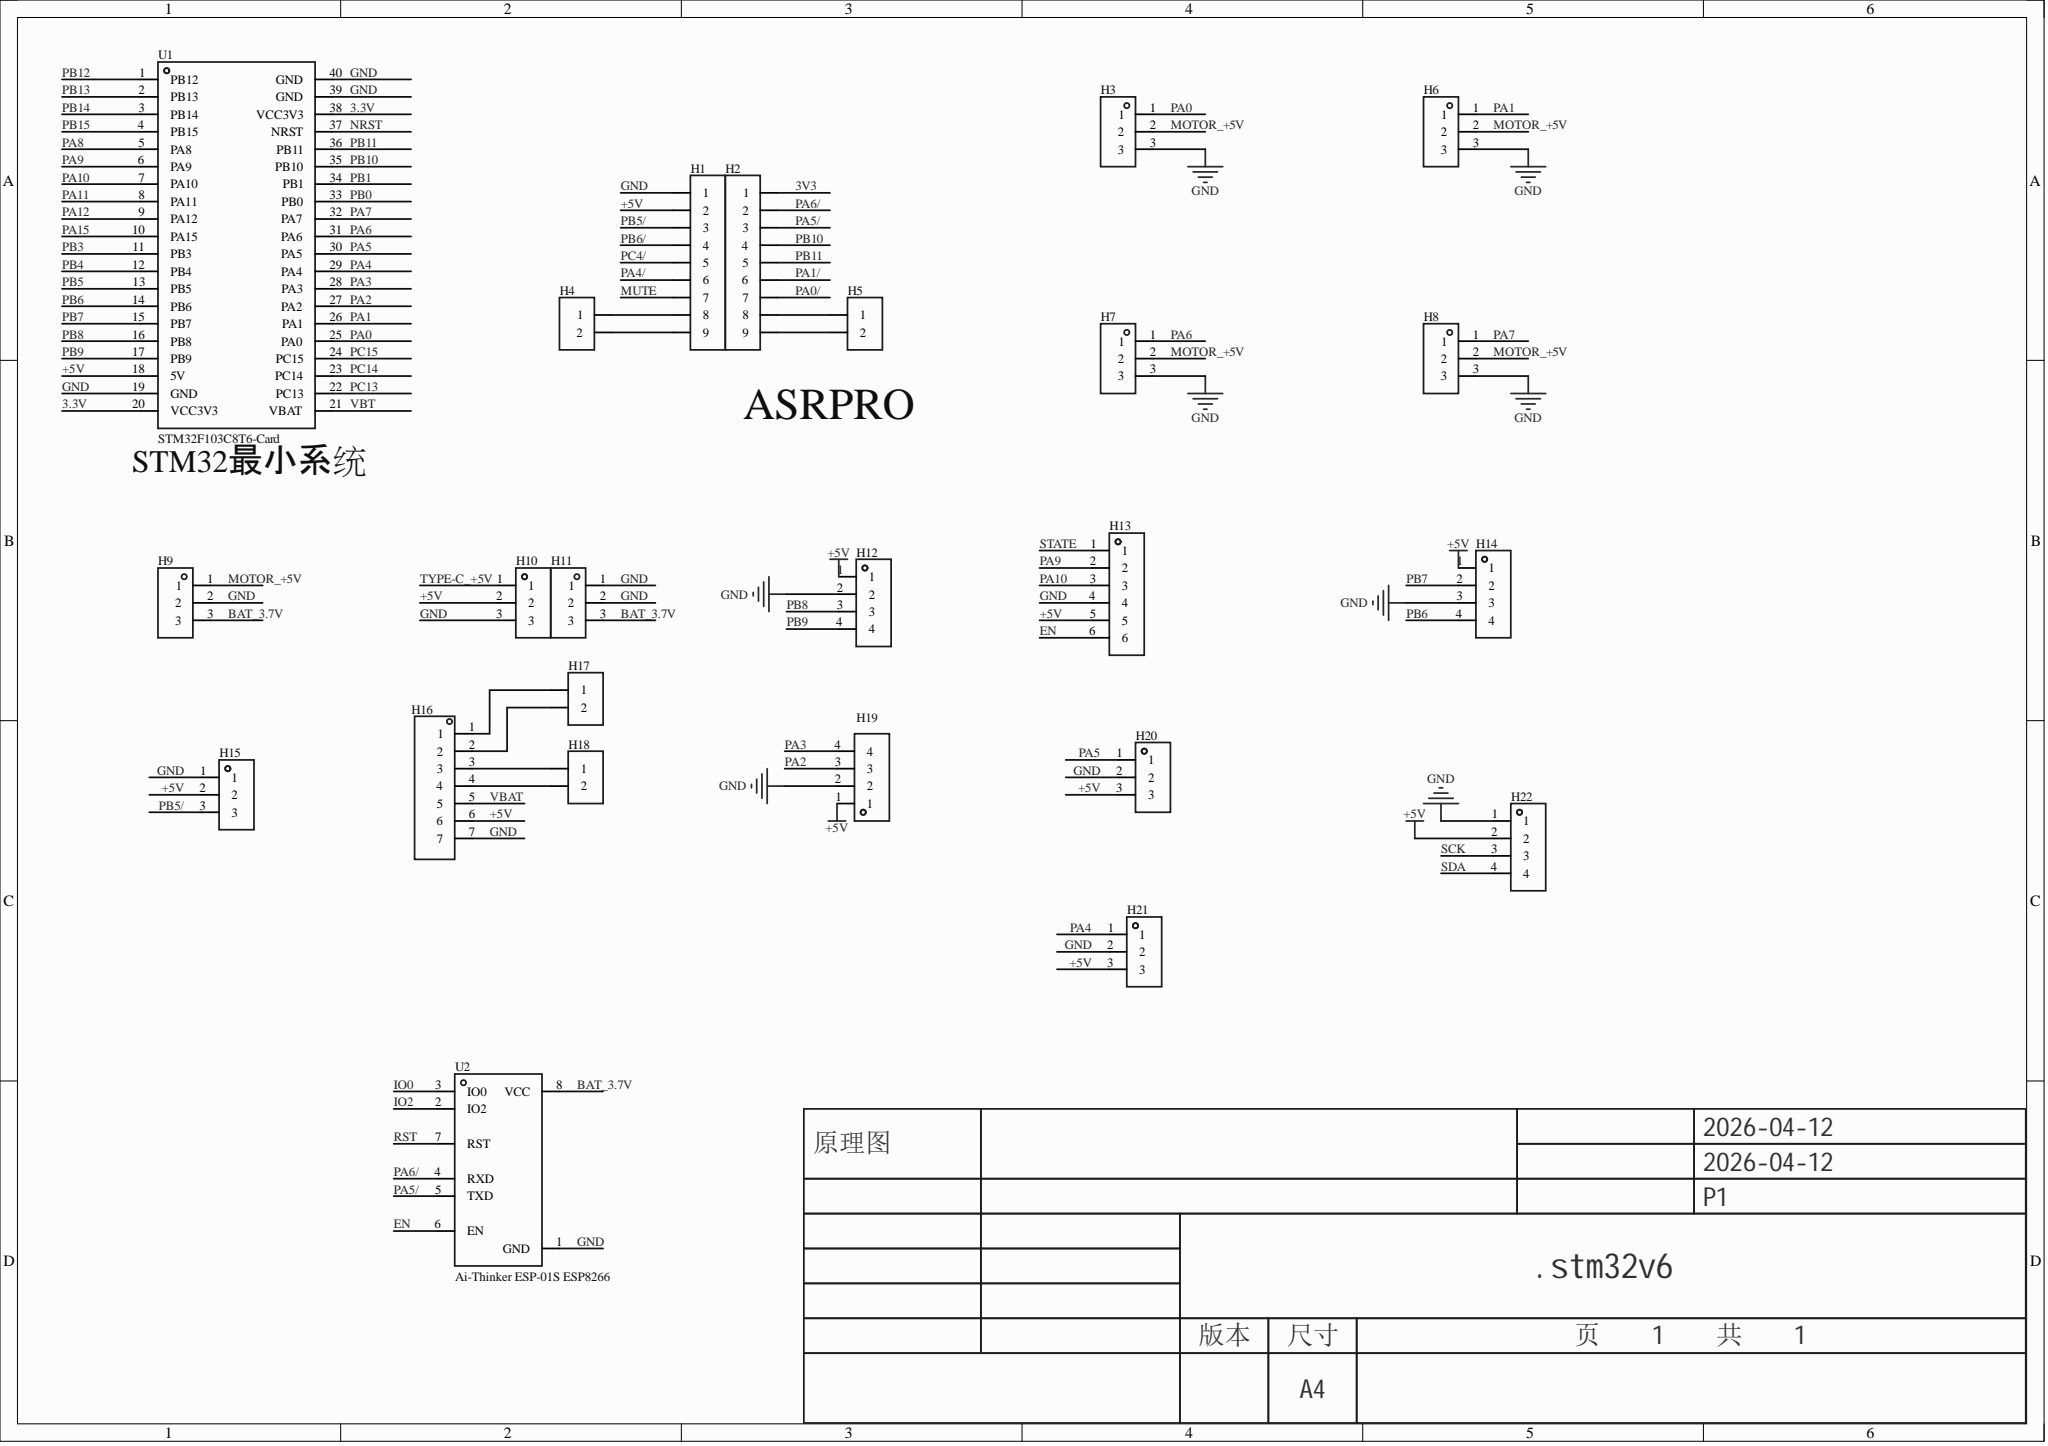Circuit board | Altium Designer | 24 parts | 33 nets
Bill of materials:
Comment,Description,Designator,Footprint,LibRef,Quantity
"","","H1, H2","HDR-TH_9P-P2.54-V-F-1","HDR-F_2.54_1x9P","2"
"","","H3, H6, H7, H8, H9, H10, H11, H15, H20, H21","HDR-TH_3P-P2.54-V-F","HDR-F_2.54_1x3P","10"
"","","H4, H5, H17, H18","HDR-TH_2P-P2.54-V-F","HDR-F_2.54_1x2P","4"
"","","H12, H14, H19, H22","HDR-TH_4P-P2.54-V-F","HDR-F_2.54_1x4P","4"
"","","H13","HDR-TH_6P-P2.54-V-F","HDR-F_2.54_1x6P","1"
"","","H16","HDR-TH_7P-P2.54-V-F","HDR-F_2.54_1x7P","1"
"STM32F103C8T6-Card","","U1","CONN-TH_L53.3-W22.9_STM32F103C8T6-CARD","STM32F103C8T6-Card","1"
"Ai-Thinker ESP-01S ESP8266","","U2","WIFIM-TH_8P-L24.7-W14.4-P2.54","Ai-Thinker ESP-01S ESP8266","1"
Netlist (Protel format):
[
H1
HDR-TH_9P-P2.54-V-F-1




]
[
H2
HDR-TH_9P-P2.54-V-F-1




]
[
H3
HDR-TH_3P-P2.54-V-F




]
[
H4
HDR-TH_2P-P2.54-V-F




]
[
H5
HDR-TH_2P-P2.54-V-F




]
[
H6
HDR-TH_3P-P2.54-V-F




]
[
H7
HDR-TH_3P-P2.54-V-F




]
[
H8
HDR-TH_3P-P2.54-V-F




]
[
H9
HDR-TH_3P-P2.54-V-F




]
[
H10
HDR-TH_3P-P2.54-V-F




]
[
H11
HDR-TH_3P-P2.54-V-F




]
[
H12
HDR-TH_4P-P2.54-V-F




]
[
H13
HDR-TH_6P-P2.54-V-F




]
[
H14
HDR-TH_4P-P2.54-V-F




]
[
H15
HDR-TH_3P-P2.54-V-F




]
[
H16
HDR-TH_7P-P2.54-V-F




]
[
H17
HDR-TH_2P-P2.54-V-F




]
[
H18
HDR-TH_2P-P2.54-V-F




]
[
H19
HDR-TH_4P-P2.54-V-F




]
[
H20
HDR-TH_3P-P2.54-V-F




]
[
H21
HDR-TH_3P-P2.54-V-F




]
[
H22
HDR-TH_4P-P2.54-V-F




]
[
U1
CONN-TH_L53.3-W22.9_STM32F103C8T6-CARD
STM32F103C8T6-Card



]
[
U2
WIFIM-TH_8P-L24.7-W14.4-P2.54
Ai-Thinker ESP-01S ESP8266



]
(
PB11
H2-5
U1-36
)
(
PB10
H2-4
U1-35
)
(
PB9
H12-4
U1-17
)
(
PB8
H12-3
U1-16
)
(
PB7
H14-2
U1-15
)
(
PB6
H14-4
U1-14
)
(
PB5/
H1-3
H15-3
)
(
PA10
H13-3
U1-7
)
(
PA9
H13-2
U1-6
)
(
PA7
H8-1
U1-32
)
(
PA6/
H2-2
U2-4
)
(
PA6
H7-1
U1-31
)
(
PA5/
H2-3
U2-5
)
(
PA5
H20-1
U1-30
)
(
PA4
H21-1
U1-29
)
(
PA3
H19-4
U1-28
)
(
PA2
H19-3
U1-27
)
(
PA1
H6-1
U1-26
)
(
PA0
H3-1
U1-25
)
(
NetH16_4
H16-4
H18-2
)
(
NetH16_3
H16-3
H18-1
)
(
NetH16_2
H16-2
H17-2
)
(
NetH16_1
H16-1
H17-1
)
(
NetH2_9
H2-9
H5-2
)
(
NetH2_8
H2-8
H5-1
)
(
NetH1_9
H1-9
H4-2
)
(
NetH1_8
H1-8
H4-1
)
(
MOTOR_+5V
H3-2
H6-2
H7-2
H8-2
H9-1
)
(
GND
H1-1
H3-3
H6-3
H7-3
H8-3
H9-2
H10-3
H11-1
H11-2
H12-2
H13-4
H14-3
H15-1
H16-7
H19-2
H20-2
H21-2
H22-1
U1-19
U1-39
U1-40
U2-1
)
(
EN
H13-6
U2-6
)
(
BAT_3.7V
H9-3
H11-3
U2-8
)
(
+5V
H1-2
H10-2
H12-1
H13-5
H14-1
H15-2
H16-6
H19-1
H20-3
H21-3
H22-2
U1-18
)
(
3.3V
U1-20
U1-38
)